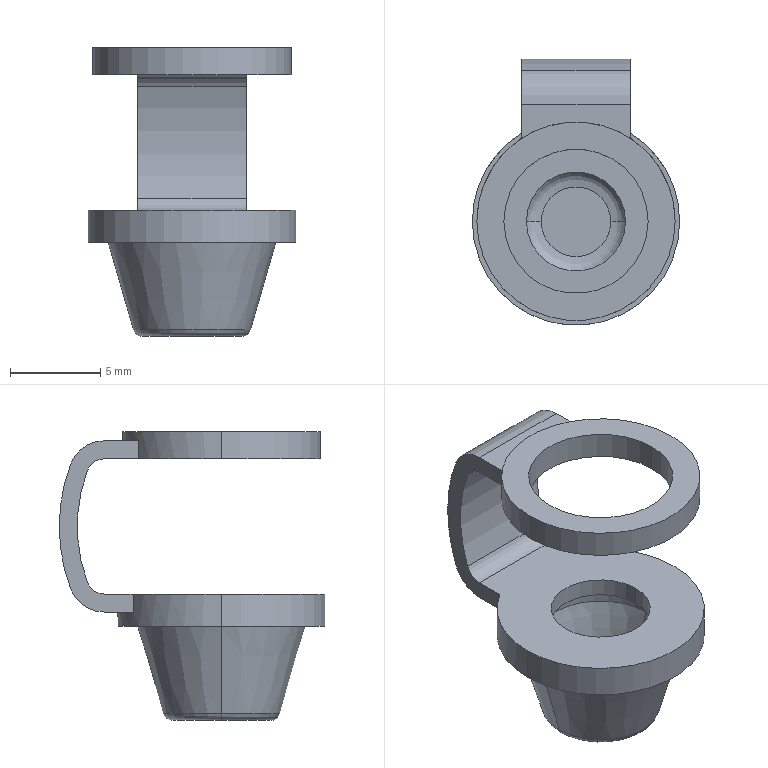Part | SolidWorks | features BaseBody 1 | 1 solid | 35 faces | box 11.5 x 14.75 x 16 mm | volume 426.893 mm3 | cylinder 16 | plane 11 | torus 4 | cone 4 | commonest cylinder face diameters 2 x2 4 x2 5.5 x2 7.1 x2 8 x2 11 x2
STEP:
#1=CARTESIAN_POINT('',(-5.5,0.,9.));
#2=VERTEX_POINT('',#1);
#3=CARTESIAN_POINT('',(-5.5,0.,7.5));
#4=VERTEX_POINT('',#3);
#5=CARTESIAN_POINT('',(-5.5,0.,2.274));
#6=DIRECTION('',(0.,0.,-1.));
#7=VECTOR('',#6,1000.);
#8=LINE('',#5,#7);
#9=EDGE_CURVE('',#2,#4,#8,.T.);
#10=ORIENTED_EDGE('',*,*,#9,.T.);
#11=CARTESIAN_POINT('',(5.5,0.,7.5));
#12=VERTEX_POINT('',#11);
#13=CARTESIAN_POINT('',(0.,0.,7.5));
#14=DIRECTION('',(0.,0.,1.));
#15=DIRECTION('',(1.,0.,0.));
#16=AXIS2_PLACEMENT_3D('',#13,#14,#15);
#17=CIRCLE('',#16,5.5);
#18=EDGE_CURVE('',#4,#12,#17,.T.);
#19=ORIENTED_EDGE('',*,*,#18,.T.);
#20=CARTESIAN_POINT('',(5.5,0.,9.));
#21=VERTEX_POINT('',#20);
#22=CARTESIAN_POINT('',(5.5,0.,2.274));
#23=DIRECTION('',(0.,0.,-1.));
#24=VECTOR('',#23,1000.);
#25=LINE('',#22,#24);
#26=EDGE_CURVE('',#21,#12,#25,.T.);
#27=ORIENTED_EDGE('',*,*,#26,.F.);
#28=CARTESIAN_POINT('',(0.,0.,9.));
#29=DIRECTION('',(0.,0.,1.));
#30=DIRECTION('',(1.,0.,0.));
#31=AXIS2_PLACEMENT_3D('',#28,#29,#30);
#32=CIRCLE('',#31,5.5);
#33=EDGE_CURVE('',#2,#21,#32,.T.);
#34=ORIENTED_EDGE('',*,*,#33,.F.);
#35=EDGE_LOOP('',(#10,#19,#27,#34));
#36=FACE_OUTER_BOUND('',#35,.T.);
#37=CARTESIAN_POINT('',(0.,0.,2.274));
#38=DIRECTION('',(0.,0.,-1.));
#39=DIRECTION('',(1.,0.,0.));
#40=AXIS2_PLACEMENT_3D('',#37,#38,#39);
#41=CYLINDRICAL_SURFACE('',#40,5.5);
#42=ADVANCED_FACE('',(#36),#41,.T.);
#43=CARTESIAN_POINT('',(4.,0.,9.));
#44=VERTEX_POINT('',#43);
#45=CARTESIAN_POINT('',(-4.,0.,9.));
#46=VERTEX_POINT('',#45);
#47=CARTESIAN_POINT('',(0.,0.,9.));
#48=DIRECTION('',(0.,0.,1.));
#49=DIRECTION('',(1.,0.,0.));
#50=AXIS2_PLACEMENT_3D('',#47,#48,#49);
#51=CIRCLE('',#50,4.);
#52=EDGE_CURVE('',#44,#46,#51,.T.);
#53=ORIENTED_EDGE('',*,*,#52,.F.);
#54=CARTESIAN_POINT('',(0.,0.,9.));
#55=DIRECTION('',(0.,0.,1.));
#56=DIRECTION('',(1.,0.,0.));
#57=AXIS2_PLACEMENT_3D('',#54,#55,#56);
#58=CIRCLE('',#57,4.);
#59=EDGE_CURVE('',#46,#44,#58,.T.);
#60=ORIENTED_EDGE('',*,*,#59,.F.);
#61=EDGE_LOOP('',(#53,#60));
#62=FACE_BOUND('',#61,.T.);
#63=CARTESIAN_POINT('',(0.,0.,9.));
#64=DIRECTION('',(0.,0.,1.));
#65=DIRECTION('',(1.,0.,0.));
#66=AXIS2_PLACEMENT_3D('',#63,#64,#65);
#67=CIRCLE('',#66,5.5);
#68=EDGE_CURVE('',#21,#2,#67,.T.);
#69=ORIENTED_EDGE('',*,*,#68,.T.);
#70=ORIENTED_EDGE('',*,*,#33,.T.);
#71=EDGE_LOOP('',(#69,#70));
#72=FACE_OUTER_BOUND('',#71,.T.);
#73=CARTESIAN_POINT('',(0.,5.5,9.));
#74=DIRECTION('',(0.,0.,-1.));
#75=DIRECTION('',(-1.,0.,0.));
#76=AXIS2_PLACEMENT_3D('',#73,#74,#75);
#77=PLANE('',#76);
#78=ADVANCED_FACE('',(#62,#72),#77,.F.);
#79=CARTESIAN_POINT('',(-4.,0.,7.5));
#80=VERTEX_POINT('',#79);
#81=CARTESIAN_POINT('',(-4.,0.,2.274));
#82=DIRECTION('',(0.,0.,-1.));
#83=VECTOR('',#82,1000.);
#84=LINE('',#81,#83);
#85=EDGE_CURVE('',#46,#80,#84,.T.);
#86=ORIENTED_EDGE('',*,*,#85,.T.);
#87=CARTESIAN_POINT('',(4.,0.,7.5));
#88=VERTEX_POINT('',#87);
#89=CARTESIAN_POINT('',(0.,0.,7.5));
#90=DIRECTION('',(0.,0.,1.));
#91=DIRECTION('',(1.,0.,0.));
#92=AXIS2_PLACEMENT_3D('',#89,#90,#91);
#93=CIRCLE('',#92,4.);
#94=EDGE_CURVE('',#88,#80,#93,.T.);
#95=ORIENTED_EDGE('',*,*,#94,.F.);
#96=CARTESIAN_POINT('',(4.,0.,2.274));
#97=DIRECTION('',(0.,0.,-1.));
#98=VECTOR('',#97,1000.);
#99=LINE('',#96,#98);
#100=EDGE_CURVE('',#44,#88,#99,.T.);
#101=ORIENTED_EDGE('',*,*,#100,.F.);
#102=ORIENTED_EDGE('',*,*,#52,.T.);
#103=EDGE_LOOP('',(#86,#95,#101,#102));
#104=FACE_OUTER_BOUND('',#103,.T.);
#105=CARTESIAN_POINT('',(0.,0.,2.274));
#106=DIRECTION('',(0.,0.,-1.));
#107=DIRECTION('',(1.,0.,0.));
#108=AXIS2_PLACEMENT_3D('',#105,#106,#107);
#109=CYLINDRICAL_SURFACE('',#108,4.);
#110=ADVANCED_FACE('',(#104),#109,.F.);
#111=CARTESIAN_POINT('',(-3.,6.5,0.));
#112=VERTEX_POINT('',#111);
#113=CARTESIAN_POINT('',(3.,6.5,0.));
#114=VERTEX_POINT('',#113);
#115=CARTESIAN_POINT('',(-3.,6.5,0.));
#116=DIRECTION('',(1.,0.,0.));
#117=VECTOR('',#116,1000.);
#118=LINE('',#115,#117);
#119=EDGE_CURVE('',#112,#114,#118,.T.);
#120=ORIENTED_EDGE('',*,*,#119,.T.);
#121=CARTESIAN_POINT('',(3.,7.436,0.648));
#122=VERTEX_POINT('',#121);
#123=CARTESIAN_POINT('',(3.,6.5,1.));
#124=DIRECTION('',(1.,0.,0.));
#125=DIRECTION('',(0.,0.,-1.));
#126=AXIS2_PLACEMENT_3D('',#123,#124,#125);
#127=CIRCLE('',#126,1.);
#128=EDGE_CURVE('',#114,#122,#127,.T.);
#129=ORIENTED_EDGE('',*,*,#128,.T.);
#130=CARTESIAN_POINT('',(-3.,7.436,0.648));
#131=VERTEX_POINT('',#130);
#132=CARTESIAN_POINT('',(-3.,7.436,0.648));
#133=DIRECTION('',(1.,0.,0.));
#134=VECTOR('',#133,1000.);
#135=LINE('',#132,#134);
#136=EDGE_CURVE('',#131,#122,#135,.T.);
#137=ORIENTED_EDGE('',*,*,#136,.F.);
#138=CARTESIAN_POINT('',(-3.,6.5,1.));
#139=DIRECTION('',(1.,0.,0.));
#140=DIRECTION('',(0.,0.,-1.));
#141=AXIS2_PLACEMENT_3D('',#138,#139,#140);
#142=CIRCLE('',#141,1.);
#143=EDGE_CURVE('',#112,#131,#142,.T.);
#144=ORIENTED_EDGE('',*,*,#143,.F.);
#145=EDGE_LOOP('',(#120,#129,#137,#144));
#146=FACE_OUTER_BOUND('',#145,.T.);
#147=CARTESIAN_POINT('',(0.,6.5,1.));
#148=DIRECTION('',(-1.,0.,0.));
#149=DIRECTION('',(0.,0.,-1.));
#150=AXIS2_PLACEMENT_3D('',#147,#148,#149);
#151=CYLINDRICAL_SURFACE('',#150,1.);
#152=ADVANCED_FACE('',(#146),#151,.F.);
#153=CARTESIAN_POINT('',(3.,6.5,-1.));
#154=VERTEX_POINT('',#153);
#155=CARTESIAN_POINT('',(-3.,6.5,-1.));
#156=VERTEX_POINT('',#155);
#157=CARTESIAN_POINT('',(-3.,6.5,-1.));
#158=DIRECTION('',(-1.,0.,0.));
#159=VECTOR('',#158,1000.);
#160=LINE('',#157,#159);
#161=EDGE_CURVE('',#154,#156,#160,.T.);
#162=ORIENTED_EDGE('',*,*,#161,.T.);
#163=CARTESIAN_POINT('',(-3.,8.372,0.296));
#164=VERTEX_POINT('',#163);
#165=CARTESIAN_POINT('',(-3.,6.5,1.));
#166=DIRECTION('',(1.,0.,0.));
#167=DIRECTION('',(0.,0.,-1.));
#168=AXIS2_PLACEMENT_3D('',#165,#166,#167);
#169=CIRCLE('',#168,2.);
#170=EDGE_CURVE('',#156,#164,#169,.T.);
#171=ORIENTED_EDGE('',*,*,#170,.T.);
#172=CARTESIAN_POINT('',(3.,8.372,0.296));
#173=VERTEX_POINT('',#172);
#174=CARTESIAN_POINT('',(-3.,8.372,0.296));
#175=DIRECTION('',(-1.,0.,0.));
#176=VECTOR('',#175,1000.);
#177=LINE('',#174,#176);
#178=EDGE_CURVE('',#173,#164,#177,.T.);
#179=ORIENTED_EDGE('',*,*,#178,.F.);
#180=CARTESIAN_POINT('',(3.,6.5,1.));
#181=DIRECTION('',(1.,0.,0.));
#182=DIRECTION('',(0.,0.,-1.));
#183=AXIS2_PLACEMENT_3D('',#180,#181,#182);
#184=CIRCLE('',#183,2.);
#185=EDGE_CURVE('',#154,#173,#184,.T.);
#186=ORIENTED_EDGE('',*,*,#185,.F.);
#187=EDGE_LOOP('',(#162,#171,#179,#186));
#188=FACE_OUTER_BOUND('',#187,.T.);
#189=CARTESIAN_POINT('',(0.,6.5,1.));
#190=DIRECTION('',(-1.,0.,0.));
#191=DIRECTION('',(0.,0.,-1.));
#192=AXIS2_PLACEMENT_3D('',#189,#190,#191);
#193=CYLINDRICAL_SURFACE('',#192,2.);
#194=ADVANCED_FACE('',(#188),#193,.T.);
#195=ORIENTED_EDGE('',*,*,#136,.T.);
#196=CARTESIAN_POINT('',(3.,7.436,6.852));
#197=VERTEX_POINT('',#196);
#198=CARTESIAN_POINT('',(3.,-0.8125,3.75));
#199=DIRECTION('',(1.,0.,0.));
#200=DIRECTION('',(0.,0.,-1.));
#201=AXIS2_PLACEMENT_3D('',#198,#199,#200);
#202=CIRCLE('',#201,8.812);
#203=EDGE_CURVE('',#122,#197,#202,.T.);
#204=ORIENTED_EDGE('',*,*,#203,.T.);
#205=CARTESIAN_POINT('',(-3.,7.436,6.852));
#206=VERTEX_POINT('',#205);
#207=CARTESIAN_POINT('',(-3.,7.436,6.852));
#208=DIRECTION('',(1.,0.,0.));
#209=VECTOR('',#208,1000.);
#210=LINE('',#207,#209);
#211=EDGE_CURVE('',#206,#197,#210,.T.);
#212=ORIENTED_EDGE('',*,*,#211,.F.);
#213=CARTESIAN_POINT('',(-3.,-0.8125,3.75));
#214=DIRECTION('',(1.,0.,0.));
#215=DIRECTION('',(0.,0.,-1.));
#216=AXIS2_PLACEMENT_3D('',#213,#214,#215);
#217=CIRCLE('',#216,8.812);
#218=EDGE_CURVE('',#131,#206,#217,.T.);
#219=ORIENTED_EDGE('',*,*,#218,.F.);
#220=EDGE_LOOP('',(#195,#204,#212,#219));
#221=FACE_OUTER_BOUND('',#220,.T.);
#222=CARTESIAN_POINT('',(0.,-0.8125,3.75));
#223=DIRECTION('',(-1.,0.,0.));
#224=DIRECTION('',(0.,0.,-1.));
#225=AXIS2_PLACEMENT_3D('',#222,#223,#224);
#226=CYLINDRICAL_SURFACE('',#225,8.812);
#227=ADVANCED_FACE('',(#221),#226,.F.);
#228=ORIENTED_EDGE('',*,*,#178,.T.);
#229=CARTESIAN_POINT('',(-3.,8.372,7.204));
#230=VERTEX_POINT('',#229);
#231=CARTESIAN_POINT('',(-3.,-0.8125,3.75));
#232=DIRECTION('',(1.,0.,0.));
#233=DIRECTION('',(0.,0.,-1.));
#234=AXIS2_PLACEMENT_3D('',#231,#232,#233);
#235=CIRCLE('',#234,9.812);
#236=EDGE_CURVE('',#164,#230,#235,.T.);
#237=ORIENTED_EDGE('',*,*,#236,.T.);
#238=CARTESIAN_POINT('',(3.,8.372,7.204));
#239=VERTEX_POINT('',#238);
#240=CARTESIAN_POINT('',(-3.,8.372,7.204));
#241=DIRECTION('',(-1.,0.,0.));
#242=VECTOR('',#241,1000.);
#243=LINE('',#240,#242);
#244=EDGE_CURVE('',#239,#230,#243,.T.);
#245=ORIENTED_EDGE('',*,*,#244,.F.);
#246=CARTESIAN_POINT('',(3.,-0.8125,3.75));
#247=DIRECTION('',(1.,0.,0.));
#248=DIRECTION('',(0.,0.,-1.));
#249=AXIS2_PLACEMENT_3D('',#246,#247,#248);
#250=CIRCLE('',#249,9.812);
#251=EDGE_CURVE('',#173,#239,#250,.T.);
#252=ORIENTED_EDGE('',*,*,#251,.F.);
#253=EDGE_LOOP('',(#228,#237,#245,#252));
#254=FACE_OUTER_BOUND('',#253,.T.);
#255=CARTESIAN_POINT('',(0.,-0.8125,3.75));
#256=DIRECTION('',(-1.,0.,0.));
#257=DIRECTION('',(0.,0.,-1.));
#258=AXIS2_PLACEMENT_3D('',#255,#256,#257);
#259=CYLINDRICAL_SURFACE('',#258,9.812);
#260=ADVANCED_FACE('',(#254),#259,.T.);
#261=ORIENTED_EDGE('',*,*,#211,.T.);
#262=CARTESIAN_POINT('',(3.,6.5,7.5));
#263=VERTEX_POINT('',#262);
#264=CARTESIAN_POINT('',(3.,6.5,6.5));
#265=DIRECTION('',(1.,0.,0.));
#266=DIRECTION('',(0.,0.,-1.));
#267=AXIS2_PLACEMENT_3D('',#264,#265,#266);
#268=CIRCLE('',#267,1.);
#269=EDGE_CURVE('',#197,#263,#268,.T.);
#270=ORIENTED_EDGE('',*,*,#269,.T.);
#271=CARTESIAN_POINT('',(-3.,6.5,7.5));
#272=VERTEX_POINT('',#271);
#273=CARTESIAN_POINT('',(-3.,6.5,7.5));
#274=DIRECTION('',(1.,0.,0.));
#275=VECTOR('',#274,1000.);
#276=LINE('',#273,#275);
#277=EDGE_CURVE('',#272,#263,#276,.T.);
#278=ORIENTED_EDGE('',*,*,#277,.F.);
#279=CARTESIAN_POINT('',(-3.,6.5,6.5));
#280=DIRECTION('',(1.,0.,0.));
#281=DIRECTION('',(0.,0.,-1.));
#282=AXIS2_PLACEMENT_3D('',#279,#280,#281);
#283=CIRCLE('',#282,1.);
#284=EDGE_CURVE('',#206,#272,#283,.T.);
#285=ORIENTED_EDGE('',*,*,#284,.F.);
#286=EDGE_LOOP('',(#261,#270,#278,#285));
#287=FACE_OUTER_BOUND('',#286,.T.);
#288=CARTESIAN_POINT('',(0.,6.5,6.5));
#289=DIRECTION('',(-1.,0.,0.));
#290=DIRECTION('',(0.,0.,-1.));
#291=AXIS2_PLACEMENT_3D('',#288,#289,#290);
#292=CYLINDRICAL_SURFACE('',#291,1.);
#293=ADVANCED_FACE('',(#287),#292,.F.);
#294=ORIENTED_EDGE('',*,*,#244,.T.);
#295=CARTESIAN_POINT('',(-3.,6.5,8.5));
#296=VERTEX_POINT('',#295);
#297=CARTESIAN_POINT('',(-3.,6.5,6.5));
#298=DIRECTION('',(1.,0.,0.));
#299=DIRECTION('',(0.,0.,-1.));
#300=AXIS2_PLACEMENT_3D('',#297,#298,#299);
#301=CIRCLE('',#300,2.);
#302=EDGE_CURVE('',#230,#296,#301,.T.);
#303=ORIENTED_EDGE('',*,*,#302,.T.);
#304=CARTESIAN_POINT('',(3.,6.5,8.5));
#305=VERTEX_POINT('',#304);
#306=CARTESIAN_POINT('',(-3.,6.5,8.5));
#307=DIRECTION('',(-1.,0.,0.));
#308=VECTOR('',#307,1000.);
#309=LINE('',#306,#308);
#310=EDGE_CURVE('',#305,#296,#309,.T.);
#311=ORIENTED_EDGE('',*,*,#310,.F.);
#312=CARTESIAN_POINT('',(3.,6.5,6.5));
#313=DIRECTION('',(1.,0.,0.));
#314=DIRECTION('',(0.,0.,-1.));
#315=AXIS2_PLACEMENT_3D('',#312,#313,#314);
#316=CIRCLE('',#315,2.);
#317=EDGE_CURVE('',#239,#305,#316,.T.);
#318=ORIENTED_EDGE('',*,*,#317,.F.);
#319=EDGE_LOOP('',(#294,#303,#311,#318));
#320=FACE_OUTER_BOUND('',#319,.T.);
#321=CARTESIAN_POINT('',(0.,6.5,6.5));
#322=DIRECTION('',(-1.,0.,0.));
#323=DIRECTION('',(0.,0.,-1.));
#324=AXIS2_PLACEMENT_3D('',#321,#322,#323);
#325=CYLINDRICAL_SURFACE('',#324,2.);
#326=ADVANCED_FACE('',(#320),#325,.T.);
#327=ORIENTED_EDGE('',*,*,#94,.T.);
#328=CARTESIAN_POINT('',(0.,0.,7.5));
#329=DIRECTION('',(0.,0.,1.));
#330=DIRECTION('',(1.,0.,0.));
#331=AXIS2_PLACEMENT_3D('',#328,#329,#330);
#332=CIRCLE('',#331,4.);
#333=EDGE_CURVE('',#80,#88,#332,.T.);
#334=ORIENTED_EDGE('',*,*,#333,.T.);
#335=EDGE_LOOP('',(#327,#334));
#336=FACE_BOUND('',#335,.T.);
#337=CARTESIAN_POINT('',(-3.,4.61,7.5));
#338=VERTEX_POINT('',#337);
#339=CARTESIAN_POINT('',(0.,0.,7.5));
#340=DIRECTION('',(0.,0.,1.));
#341=DIRECTION('',(1.,0.,0.));
#342=AXIS2_PLACEMENT_3D('',#339,#340,#341);
#343=CIRCLE('',#342,5.5);
#344=EDGE_CURVE('',#338,#4,#343,.T.);
#345=ORIENTED_EDGE('',*,*,#344,.F.);
#346=CARTESIAN_POINT('',(-3.,6.5,7.5));
#347=DIRECTION('',(0.,-1.,0.));
#348=VECTOR('',#347,1000.);
#349=LINE('',#346,#348);
#350=EDGE_CURVE('',#272,#338,#349,.T.);
#351=ORIENTED_EDGE('',*,*,#350,.F.);
#352=ORIENTED_EDGE('',*,*,#277,.T.);
#353=CARTESIAN_POINT('',(3.,4.61,7.5));
#354=VERTEX_POINT('',#353);
#355=CARTESIAN_POINT('',(3.,6.5,7.5));
#356=DIRECTION('',(0.,-1.,0.));
#357=VECTOR('',#356,1000.);
#358=LINE('',#355,#357);
#359=EDGE_CURVE('',#263,#354,#358,.T.);
#360=ORIENTED_EDGE('',*,*,#359,.T.);
#361=CARTESIAN_POINT('',(0.,0.,7.5));
#362=DIRECTION('',(0.,0.,1.));
#363=DIRECTION('',(1.,0.,0.));
#364=AXIS2_PLACEMENT_3D('',#361,#362,#363);
#365=CIRCLE('',#364,5.5);
#366=EDGE_CURVE('',#12,#354,#365,.T.);
#367=ORIENTED_EDGE('',*,*,#366,.F.);
#368=ORIENTED_EDGE('',*,*,#18,.F.);
#369=EDGE_LOOP('',(#345,#351,#352,#360,#367,#368));
#370=FACE_OUTER_BOUND('',#369,.T.);
#371=CARTESIAN_POINT('',(-3.,6.5,7.5));
#372=DIRECTION('',(0.,0.,1.));
#373=DIRECTION('',(1.,0.,0.));
#374=AXIS2_PLACEMENT_3D('',#371,#372,#373);
#375=PLANE('',#374);
#376=ADVANCED_FACE('',(#336,#370),#375,.F.);
#377=CARTESIAN_POINT('',(3.,4.905,-1.));
#378=VERTEX_POINT('',#377);
#379=CARTESIAN_POINT('',(-3.,4.905,-1.));
#380=VERTEX_POINT('',#379);
#381=CARTESIAN_POINT('',(0.,0.,-1.));
#382=DIRECTION('',(0.,0.,1.));
#383=DIRECTION('',(0.,-1.,0.));
#384=AXIS2_PLACEMENT_3D('',#381,#382,#383);
#385=CIRCLE('',#384,5.75);
#386=EDGE_CURVE('',#378,#380,#385,.T.);
#387=ORIENTED_EDGE('',*,*,#386,.T.);
#388=CARTESIAN_POINT('',(-3.,6.5,-1.));
#389=DIRECTION('',(0.,-1.,0.));
#390=VECTOR('',#389,1000.);
#391=LINE('',#388,#390);
#392=EDGE_CURVE('',#156,#380,#391,.T.);
#393=ORIENTED_EDGE('',*,*,#392,.F.);
#394=ORIENTED_EDGE('',*,*,#161,.F.);
#395=CARTESIAN_POINT('',(3.,6.5,-1.));
#396=DIRECTION('',(0.,-1.,0.));
#397=VECTOR('',#396,1000.);
#398=LINE('',#395,#397);
#399=EDGE_CURVE('',#154,#378,#398,.T.);
#400=ORIENTED_EDGE('',*,*,#399,.T.);
#401=EDGE_LOOP('',(#387,#393,#394,#400));
#402=FACE_OUTER_BOUND('',#401,.T.);
#403=CARTESIAN_POINT('',(-3.,6.5,-1.));
#404=DIRECTION('',(0.,0.,-1.));
#405=DIRECTION('',(-1.,0.,0.));
#406=AXIS2_PLACEMENT_3D('',#403,#404,#405);
#407=PLANE('',#406);
#408=ADVANCED_FACE('',(#402),#407,.T.);
#409=CARTESIAN_POINT('',(1.931,0.,-5.));
#410=VERTEX_POINT('',#409);
#411=CARTESIAN_POINT('',(-1.931,0.,-5.));
#412=VERTEX_POINT('',#411);
#413=CARTESIAN_POINT('',(0.,0.,-5.));
#414=DIRECTION('',(0.,0.,1.));
#415=DIRECTION('',(1.,0.,0.));
#416=AXIS2_PLACEMENT_3D('',#413,#414,#415);
#417=CIRCLE('',#416,1.931);
#418=EDGE_CURVE('',#410,#412,#417,.T.);
#419=ORIENTED_EDGE('',*,*,#418,.T.);
#420=CARTESIAN_POINT('',(0.,0.,-5.));
#421=DIRECTION('',(0.,0.,1.));
#422=DIRECTION('',(1.,0.,0.));
#423=AXIS2_PLACEMENT_3D('',#420,#421,#422);
#424=CIRCLE('',#423,1.931);
#425=EDGE_CURVE('',#412,#410,#424,.T.);
#426=ORIENTED_EDGE('',*,*,#425,.T.);
#427=EDGE_LOOP('',(#419,#426));
#428=FACE_OUTER_BOUND('',#427,.T.);
#429=CARTESIAN_POINT('',(0.,1.931,-5.));
#430=DIRECTION('',(0.,0.,-1.));
#431=DIRECTION('',(-1.,0.,0.));
#432=AXIS2_PLACEMENT_3D('',#429,#430,#431);
#433=PLANE('',#432);
#434=ADVANCED_FACE('',(#428),#433,.F.);
#435=CARTESIAN_POINT('',(-2.892,0.,-4.278));
#436=VERTEX_POINT('',#435);
#437=CARTESIAN_POINT('',(-1.931,0.,-4.));
#438=DIRECTION('',(0.,-1.,0.));
#439=DIRECTION('',(-1.,0.,0.));
#440=AXIS2_PLACEMENT_3D('',#437,#438,#439);
#441=CIRCLE('',#440,1.);
#442=EDGE_CURVE('',#436,#412,#441,.T.);
#443=ORIENTED_EDGE('',*,*,#442,.T.);
#444=ORIENTED_EDGE('',*,*,#418,.F.);
#445=CARTESIAN_POINT('',(2.892,0.,-4.278));
#446=VERTEX_POINT('',#445);
#447=CARTESIAN_POINT('',(1.931,0.,-4.));
#448=DIRECTION('',(0.,1.,0.));
#449=DIRECTION('',(1.,0.,0.));
#450=AXIS2_PLACEMENT_3D('',#447,#448,#449);
#451=CIRCLE('',#450,1.);
#452=EDGE_CURVE('',#446,#410,#451,.T.);
#453=ORIENTED_EDGE('',*,*,#452,.F.);
#454=CARTESIAN_POINT('',(0.,0.,-4.278));
#455=DIRECTION('',(0.,0.,1.));
#456=DIRECTION('',(1.,0.,0.));
#457=AXIS2_PLACEMENT_3D('',#454,#455,#456);
#458=CIRCLE('',#457,2.892);
#459=EDGE_CURVE('',#446,#436,#458,.T.);
#460=ORIENTED_EDGE('',*,*,#459,.T.);
#461=EDGE_LOOP('',(#443,#444,#453,#460));
#462=FACE_OUTER_BOUND('',#461,.T.);
#463=CARTESIAN_POINT('',(0.,0.,-4.));
#464=DIRECTION('',(0.,0.,-1.));
#465=DIRECTION('',(1.,0.,0.));
#466=AXIS2_PLACEMENT_3D('',#463,#464,#465);
#467=TOROIDAL_SURFACE('',#466,1.931,1.);
#468=ADVANCED_FACE('',(#462),#467,.F.);
#469=CARTESIAN_POINT('',(3.55,0.,-2.));
#470=VERTEX_POINT('',#469);
#471=CARTESIAN_POINT('',(2.892,0.,-4.278));
#472=DIRECTION('',(0.2777,0.,0.9607));
#473=VECTOR('',#472,1000.);
#474=LINE('',#471,#473);
#475=EDGE_CURVE('',#446,#470,#474,.T.);
#476=ORIENTED_EDGE('',*,*,#475,.T.);
#477=CARTESIAN_POINT('',(-3.55,0.,-2.));
#478=VERTEX_POINT('',#477);
#479=CARTESIAN_POINT('',(0.,0.,-2.));
#480=DIRECTION('',(0.,0.,1.));
#481=DIRECTION('',(1.,0.,0.));
#482=AXIS2_PLACEMENT_3D('',#479,#480,#481);
#483=CIRCLE('',#482,3.55);
#484=EDGE_CURVE('',#470,#478,#483,.T.);
#485=ORIENTED_EDGE('',*,*,#484,.T.);
#486=CARTESIAN_POINT('',(-2.892,0.,-4.278));
#487=DIRECTION('',(-0.2777,0.,0.9607));
#488=VECTOR('',#487,1000.);
#489=LINE('',#486,#488);
#490=EDGE_CURVE('',#436,#478,#489,.T.);
#491=ORIENTED_EDGE('',*,*,#490,.F.);
#492=ORIENTED_EDGE('',*,*,#459,.F.);
#493=EDGE_LOOP('',(#476,#485,#491,#492));
#494=FACE_OUTER_BOUND('',#493,.T.);
#495=CARTESIAN_POINT('',(0.,0.,-4.278));
#496=DIRECTION('',(0.,0.,1.));
#497=DIRECTION('',(-1.,0.,0.));
#498=AXIS2_PLACEMENT_3D('',#495,#496,#497);
#499=CONICAL_SURFACE('',#498,2.892,0.2814);
#500=ADVANCED_FACE('',(#494),#499,.F.);
#501=CARTESIAN_POINT('',(-3.55,0.,-1.));
#502=VERTEX_POINT('',#501);
#503=CARTESIAN_POINT('',(-3.55,0.,0.));
#504=DIRECTION('',(0.,0.,-1.));
#505=VECTOR('',#504,1000.);
#506=LINE('',#503,#505);
#507=EDGE_CURVE('',#502,#478,#506,.T.);
#508=ORIENTED_EDGE('',*,*,#507,.T.);
#509=ORIENTED_EDGE('',*,*,#484,.F.);
#510=CARTESIAN_POINT('',(3.55,0.,-1.));
#511=VERTEX_POINT('',#510);
#512=CARTESIAN_POINT('',(3.55,0.,0.));
#513=DIRECTION('',(0.,0.,-1.));
#514=VECTOR('',#513,1000.);
#515=LINE('',#512,#514);
#516=EDGE_CURVE('',#511,#470,#515,.T.);
#517=ORIENTED_EDGE('',*,*,#516,.F.);
#518=CARTESIAN_POINT('',(0.,0.,-1.));
#519=DIRECTION('',(0.,0.,1.));
#520=DIRECTION('',(1.,0.,0.));
#521=AXIS2_PLACEMENT_3D('',#518,#519,#520);
#522=CIRCLE('',#521,3.55);
#523=EDGE_CURVE('',#511,#502,#522,.T.);
#524=ORIENTED_EDGE('',*,*,#523,.T.);
#525=EDGE_LOOP('',(#508,#509,#517,#524));
#526=FACE_OUTER_BOUND('',#525,.T.);
#527=CARTESIAN_POINT('',(0.,0.,0.));
#528=DIRECTION('',(0.,0.,-1.));
#529=DIRECTION('',(1.,0.,0.));
#530=AXIS2_PLACEMENT_3D('',#527,#528,#529);
#531=CYLINDRICAL_SURFACE('',#530,3.55);
#532=ADVANCED_FACE('',(#526),#531,.F.);
#533=CARTESIAN_POINT('',(2.75,0.,-1.));
#534=VERTEX_POINT('',#533);
#535=CARTESIAN_POINT('',(-2.75,0.,-1.));
#536=VERTEX_POINT('',#535);
#537=CARTESIAN_POINT('',(0.,0.,-1.));
#538=DIRECTION('',(0.,0.,1.));
#539=DIRECTION('',(1.,0.,0.));
#540=AXIS2_PLACEMENT_3D('',#537,#538,#539);
#541=CIRCLE('',#540,2.75);
#542=EDGE_CURVE('',#534,#536,#541,.T.);
#543=ORIENTED_EDGE('',*,*,#542,.T.);
#544=CARTESIAN_POINT('',(0.,0.,-1.));
#545=DIRECTION('',(0.,0.,1.));
#546=DIRECTION('',(1.,0.,0.));
#547=AXIS2_PLACEMENT_3D('',#544,#545,#546);
#548=CIRCLE('',#547,2.75);
#549=EDGE_CURVE('',#536,#534,#548,.T.);
#550=ORIENTED_EDGE('',*,*,#549,.T.);
#551=EDGE_LOOP('',(#543,#550));
#552=FACE_BOUND('',#551,.T.);
#553=ORIENTED_EDGE('',*,*,#523,.F.);
#554=CARTESIAN_POINT('',(0.,0.,-1.));
#555=DIRECTION('',(0.,0.,1.));
#556=DIRECTION('',(1.,0.,0.));
#557=AXIS2_PLACEMENT_3D('',#554,#555,#556);
#558=CIRCLE('',#557,3.55);
#559=EDGE_CURVE('',#502,#511,#558,.T.);
#560=ORIENTED_EDGE('',*,*,#559,.F.);
#561=EDGE_LOOP('',(#553,#560));
#562=FACE_OUTER_BOUND('',#561,.T.);
#563=CARTESIAN_POINT('',(0.,2.75,-1.));
#564=DIRECTION('',(0.,0.,1.));
#565=DIRECTION('',(1.,0.,0.));
#566=AXIS2_PLACEMENT_3D('',#563,#564,#565);
#567=PLANE('',#566);
#568=ADVANCED_FACE('',(#552,#562),#567,.F.);
#569=CARTESIAN_POINT('',(-2.75,0.,0.));
#570=VERTEX_POINT('',#569);
#571=CARTESIAN_POINT('',(-2.75,0.,0.));
#572=DIRECTION('',(0.,0.,-1.));
#573=VECTOR('',#572,1000.);
#574=LINE('',#571,#573);
#575=EDGE_CURVE('',#570,#536,#574,.T.);
#576=ORIENTED_EDGE('',*,*,#575,.T.);
#577=ORIENTED_EDGE('',*,*,#542,.F.);
#578=CARTESIAN_POINT('',(2.75,0.,0.));
#579=VERTEX_POINT('',#578);
#580=CARTESIAN_POINT('',(2.75,0.,0.));
#581=DIRECTION('',(0.,0.,-1.));
#582=VECTOR('',#581,1000.);
#583=LINE('',#580,#582);
#584=EDGE_CURVE('',#579,#534,#583,.T.);
#585=ORIENTED_EDGE('',*,*,#584,.F.);
#586=CARTESIAN_POINT('',(0.,0.,0.));
#587=DIRECTION('',(0.,0.,1.));
#588=DIRECTION('',(1.,0.,0.));
#589=AXIS2_PLACEMENT_3D('',#586,#587,#588);
#590=CIRCLE('',#589,2.75);
#591=EDGE_CURVE('',#579,#570,#590,.T.);
#592=ORIENTED_EDGE('',*,*,#591,.T.);
#593=EDGE_LOOP('',(#576,#577,#585,#592));
#594=FACE_OUTER_BOUND('',#593,.T.);
#595=CARTESIAN_POINT('',(0.,0.,0.));
#596=DIRECTION('',(0.,0.,-1.));
#597=DIRECTION('',(1.,0.,0.));
#598=AXIS2_PLACEMENT_3D('',#595,#596,#597);
#599=CYLINDRICAL_SURFACE('',#598,2.75);
#600=ADVANCED_FACE('',(#594),#599,.F.);
#601=ORIENTED_EDGE('',*,*,#591,.F.);
#602=CARTESIAN_POINT('',(0.,0.,0.));
#603=DIRECTION('',(0.,0.,1.));
#604=DIRECTION('',(1.,0.,0.));
#605=AXIS2_PLACEMENT_3D('',#602,#603,#604);
#606=CIRCLE('',#605,2.75);
#607=EDGE_CURVE('',#570,#579,#606,.T.);
#608=ORIENTED_EDGE('',*,*,#607,.F.);
#609=EDGE_LOOP('',(#601,#608));
#610=FACE_BOUND('',#609,.T.);
#611=CARTESIAN_POINT('',(-3.,4.905,0.));
#612=VERTEX_POINT('',#611);
#613=CARTESIAN_POINT('',(-5.75,0.,0.));
#614=VERTEX_POINT('',#613);
#615=CARTESIAN_POINT('',(0.,0.,0.));
#616=DIRECTION('',(0.,0.,1.));
#617=DIRECTION('',(1.,0.,0.));
#618=AXIS2_PLACEMENT_3D('',#615,#616,#617);
#619=CIRCLE('',#618,5.75);
#620=EDGE_CURVE('',#612,#614,#619,.T.);
#621=ORIENTED_EDGE('',*,*,#620,.T.);
#622=CARTESIAN_POINT('',(5.75,0.,0.));
#623=VERTEX_POINT('',#622);
#624=CARTESIAN_POINT('',(0.,0.,0.));
#625=DIRECTION('',(0.,0.,1.));
#626=DIRECTION('',(1.,0.,0.));
#627=AXIS2_PLACEMENT_3D('',#624,#625,#626);
#628=CIRCLE('',#627,5.75);
#629=EDGE_CURVE('',#614,#623,#628,.T.);
#630=ORIENTED_EDGE('',*,*,#629,.T.);
#631=CARTESIAN_POINT('',(3.,4.905,0.));
#632=VERTEX_POINT('',#631);
#633=CARTESIAN_POINT('',(0.,0.,0.));
#634=DIRECTION('',(0.,0.,1.));
#635=DIRECTION('',(1.,0.,0.));
#636=AXIS2_PLACEMENT_3D('',#633,#634,#635);
#637=CIRCLE('',#636,5.75);
#638=EDGE_CURVE('',#623,#632,#637,.T.);
#639=ORIENTED_EDGE('',*,*,#638,.T.);
#640=CARTESIAN_POINT('',(3.,6.5,0.));
#641=DIRECTION('',(0.,-1.,0.));
#642=VECTOR('',#641,1000.);
#643=LINE('',#640,#642);
#644=EDGE_CURVE('',#114,#632,#643,.T.);
#645=ORIENTED_EDGE('',*,*,#644,.F.);
#646=ORIENTED_EDGE('',*,*,#119,.F.);
#647=CARTESIAN_POINT('',(-3.,6.5,0.));
#648=DIRECTION('',(0.,-1.,0.));
#649=VECTOR('',#648,1000.);
#650=LINE('',#647,#649);
#651=EDGE_CURVE('',#112,#612,#650,.T.);
#652=ORIENTED_EDGE('',*,*,#651,.T.);
#653=EDGE_LOOP('',(#621,#630,#639,#645,#646,#652));
#654=FACE_OUTER_BOUND('',#653,.T.);
#655=CARTESIAN_POINT('',(0.,2.75,0.));
#656=DIRECTION('',(0.,0.,-1.));
#657=DIRECTION('',(-1.,0.,0.));
#658=AXIS2_PLACEMENT_3D('',#655,#656,#657);
#659=PLANE('',#658);
#660=ADVANCED_FACE('',(#610,#654),#659,.F.);
#661=CARTESIAN_POINT('',(-5.75,0.,-1.8));
#662=VERTEX_POINT('',#661);
#663=CARTESIAN_POINT('',(-5.75,0.,0.));
#664=DIRECTION('',(0.,0.,-1.));
#665=VECTOR('',#664,1000.);
#666=LINE('',#663,#665);
#667=EDGE_CURVE('',#614,#662,#666,.T.);
#668=ORIENTED_EDGE('',*,*,#667,.T.);
#669=CARTESIAN_POINT('',(5.75,0.,-1.8));
#670=VERTEX_POINT('',#669);
#671=CARTESIAN_POINT('',(0.,0.,-1.8));
#672=DIRECTION('',(0.,0.,1.));
#673=DIRECTION('',(1.,0.,0.));
#674=AXIS2_PLACEMENT_3D('',#671,#672,#673);
#675=CIRCLE('',#674,5.75);
#676=EDGE_CURVE('',#662,#670,#675,.T.);
#677=ORIENTED_EDGE('',*,*,#676,.T.);
#678=CARTESIAN_POINT('',(5.75,0.,0.));
#679=DIRECTION('',(0.,0.,-1.));
#680=VECTOR('',#679,1000.);
#681=LINE('',#678,#680);
#682=EDGE_CURVE('',#623,#670,#681,.T.);
#683=ORIENTED_EDGE('',*,*,#682,.F.);
#684=ORIENTED_EDGE('',*,*,#629,.F.);
#685=EDGE_LOOP('',(#668,#677,#683,#684));
#686=FACE_OUTER_BOUND('',#685,.T.);
#687=CARTESIAN_POINT('',(0.,0.,0.));
#688=DIRECTION('',(0.,0.,-1.));
#689=DIRECTION('',(1.,0.,0.));
#690=AXIS2_PLACEMENT_3D('',#687,#688,#689);
#691=CYLINDRICAL_SURFACE('',#690,5.75);
#692=ADVANCED_FACE('',(#686),#691,.T.);
#693=CARTESIAN_POINT('',(-4.649,0.,-1.8));
#694=VERTEX_POINT('',#693);
#695=CARTESIAN_POINT('',(4.649,0.,-1.8));
#696=VERTEX_POINT('',#695);
#697=CARTESIAN_POINT('',(0.,0.,-1.8));
#698=DIRECTION('',(0.,0.,1.));
#699=DIRECTION('',(1.,0.,0.));
#700=AXIS2_PLACEMENT_3D('',#697,#698,#699);
#701=CIRCLE('',#700,4.649);
#702=EDGE_CURVE('',#694,#696,#701,.T.);
#703=ORIENTED_EDGE('',*,*,#702,.T.);
#704=CARTESIAN_POINT('',(0.,0.,-1.8));
#705=DIRECTION('',(0.,0.,1.));
#706=DIRECTION('',(1.,0.,0.));
#707=AXIS2_PLACEMENT_3D('',#704,#705,#706);
#708=CIRCLE('',#707,4.649);
#709=EDGE_CURVE('',#696,#694,#708,.T.);
#710=ORIENTED_EDGE('',*,*,#709,.T.);
#711=EDGE_LOOP('',(#703,#710));
#712=FACE_BOUND('',#711,.T.);
#713=CARTESIAN_POINT('',(0.,0.,-1.8));
#714=DIRECTION('',(0.,0.,1.));
#715=DIRECTION('',(1.,0.,0.));
#716=AXIS2_PLACEMENT_3D('',#713,#714,#715);
#717=CIRCLE('',#716,5.75);
#718=EDGE_CURVE('',#670,#662,#717,.T.);
#719=ORIENTED_EDGE('',*,*,#718,.F.);
#720=ORIENTED_EDGE('',*,*,#676,.F.);
#721=EDGE_LOOP('',(#719,#720));
#722=FACE_OUTER_BOUND('',#721,.T.);
#723=CARTESIAN_POINT('',(0.,5.75,-1.8));
#724=DIRECTION('',(0.,0.,1.));
#725=DIRECTION('',(1.,0.,0.));
#726=AXIS2_PLACEMENT_3D('',#723,#724,#725);
#727=PLANE('',#726);
#728=ADVANCED_FACE('',(#712,#722),#727,.F.);
#729=CARTESIAN_POINT('',(3.25,0.,-6.639));
#730=VERTEX_POINT('',#729);
#731=CARTESIAN_POINT('',(4.649,0.,-1.8));
#732=DIRECTION('',(0.2777,0.,0.9607));
#733=VECTOR('',#732,1000.);
#734=LINE('',#731,#733);
#735=EDGE_CURVE('',#730,#696,#734,.T.);
#736=ORIENTED_EDGE('',*,*,#735,.T.);
#737=ORIENTED_EDGE('',*,*,#702,.F.);
#738=CARTESIAN_POINT('',(-3.25,0.,-6.639));
#739=VERTEX_POINT('',#738);
#740=CARTESIAN_POINT('',(-4.649,0.,-1.8));
#741=DIRECTION('',(-0.2777,0.,0.9607));
#742=VECTOR('',#741,1000.);
#743=LINE('',#740,#742);
#744=EDGE_CURVE('',#739,#694,#743,.T.);
#745=ORIENTED_EDGE('',*,*,#744,.F.);
#746=CARTESIAN_POINT('',(0.,0.,-6.639));
#747=DIRECTION('',(0.,0.,1.));
#748=DIRECTION('',(1.,0.,0.));
#749=AXIS2_PLACEMENT_3D('',#746,#747,#748);
#750=CIRCLE('',#749,3.25);
#751=EDGE_CURVE('',#739,#730,#750,.T.);
#752=ORIENTED_EDGE('',*,*,#751,.T.);
#753=EDGE_LOOP('',(#736,#737,#745,#752));
#754=FACE_OUTER_BOUND('',#753,.T.);
#755=CARTESIAN_POINT('',(0.,0.,-1.8));
#756=DIRECTION('',(0.,0.,1.));
#757=DIRECTION('',(-1.,0.,0.));
#758=AXIS2_PLACEMENT_3D('',#755,#756,#757);
#759=CONICAL_SURFACE('',#758,4.649,0.2814);
#760=ADVANCED_FACE('',(#754),#759,.T.);
#761=CARTESIAN_POINT('',(-2.77,0.,-7.));
#762=VERTEX_POINT('',#761);
#763=CARTESIAN_POINT('',(-2.77,0.,-6.5));
#764=DIRECTION('',(0.,-1.,0.));
#765=DIRECTION('',(-1.,0.,0.));
#766=AXIS2_PLACEMENT_3D('',#763,#764,#765);
#767=CIRCLE('',#766,0.5);
#768=EDGE_CURVE('',#739,#762,#767,.T.);
#769=ORIENTED_EDGE('',*,*,#768,.T.);
#770=CARTESIAN_POINT('',(2.77,0.,-7.));
#771=VERTEX_POINT('',#770);
#772=CARTESIAN_POINT('',(0.,0.,-7.));
#773=DIRECTION('',(0.,0.,1.));
#774=DIRECTION('',(1.,0.,0.));
#775=AXIS2_PLACEMENT_3D('',#772,#773,#774);
#776=CIRCLE('',#775,2.77);
#777=EDGE_CURVE('',#762,#771,#776,.T.);
#778=ORIENTED_EDGE('',*,*,#777,.T.);
#779=CARTESIAN_POINT('',(2.77,0.,-6.5));
#780=DIRECTION('',(0.,1.,0.));
#781=DIRECTION('',(1.,0.,0.));
#782=AXIS2_PLACEMENT_3D('',#779,#780,#781);
#783=CIRCLE('',#782,0.5);
#784=EDGE_CURVE('',#730,#771,#783,.T.);
#785=ORIENTED_EDGE('',*,*,#784,.F.);
#786=ORIENTED_EDGE('',*,*,#751,.F.);
#787=EDGE_LOOP('',(#769,#778,#785,#786));
#788=FACE_OUTER_BOUND('',#787,.T.);
#789=CARTESIAN_POINT('',(0.,0.,-6.5));
#790=DIRECTION('',(0.,0.,-1.));
#791=DIRECTION('',(1.,0.,0.));
#792=AXIS2_PLACEMENT_3D('',#789,#790,#791);
#793=TOROIDAL_SURFACE('',#792,2.77,0.5);
#794=ADVANCED_FACE('',(#788),#793,.T.);
#795=CARTESIAN_POINT('',(0.,0.,-7.));
#796=DIRECTION('',(0.,0.,1.));
#797=DIRECTION('',(1.,0.,0.));
#798=AXIS2_PLACEMENT_3D('',#795,#796,#797);
#799=CIRCLE('',#798,2.77);
#800=EDGE_CURVE('',#771,#762,#799,.T.);
#801=ORIENTED_EDGE('',*,*,#800,.F.);
#802=ORIENTED_EDGE('',*,*,#777,.F.);
#803=EDGE_LOOP('',(#801,#802));
#804=FACE_OUTER_BOUND('',#803,.T.);
#805=CARTESIAN_POINT('',(0.,2.77,-7.));
#806=DIRECTION('',(0.,0.,1.));
#807=DIRECTION('',(1.,0.,0.));
#808=AXIS2_PLACEMENT_3D('',#805,#806,#807);
#809=PLANE('',#808);
#810=ADVANCED_FACE('',(#804),#809,.F.);
#811=CARTESIAN_POINT('',(-3.,4.61,8.5));
#812=VERTEX_POINT('',#811);
#813=CARTESIAN_POINT('',(3.,4.61,8.5));
#814=VERTEX_POINT('',#813);
#815=CARTESIAN_POINT('',(0.,0.,8.5));
#816=DIRECTION('',(0.,0.,-1.));
#817=DIRECTION('',(1.,0.,0.));
#818=AXIS2_PLACEMENT_3D('',#815,#816,#817);
#819=CIRCLE('',#818,5.5);
#820=EDGE_CURVE('',#812,#814,#819,.T.);
#821=ORIENTED_EDGE('',*,*,#820,.T.);
#822=CARTESIAN_POINT('',(3.,6.5,8.5));
#823=DIRECTION('',(0.,-1.,0.));
#824=VECTOR('',#823,1000.);
#825=LINE('',#822,#824);
#826=EDGE_CURVE('',#305,#814,#825,.T.);
#827=ORIENTED_EDGE('',*,*,#826,.F.);
#828=ORIENTED_EDGE('',*,*,#310,.T.);
#829=CARTESIAN_POINT('',(-3.,6.5,8.5));
#830=DIRECTION('',(0.,-1.,0.));
#831=VECTOR('',#830,1000.);
#832=LINE('',#829,#831);
#833=EDGE_CURVE('',#296,#812,#832,.T.);
#834=ORIENTED_EDGE('',*,*,#833,.T.);
#835=EDGE_LOOP('',(#821,#827,#828,#834));
#836=FACE_OUTER_BOUND('',#835,.T.);
#837=CARTESIAN_POINT('',(-3.,6.5,8.5));
#838=DIRECTION('',(0.,0.,-1.));
#839=DIRECTION('',(-1.,0.,0.));
#840=AXIS2_PLACEMENT_3D('',#837,#838,#839);
#841=PLANE('',#840);
#842=ADVANCED_FACE('',(#836),#841,.F.);
#843=ORIENTED_EDGE('',*,*,#359,.F.);
#844=ORIENTED_EDGE('',*,*,#269,.F.);
#845=ORIENTED_EDGE('',*,*,#203,.F.);
#846=ORIENTED_EDGE('',*,*,#128,.F.);
#847=ORIENTED_EDGE('',*,*,#644,.T.);
#848=CARTESIAN_POINT('',(3.,4.905,0.));
#849=DIRECTION('',(0.,0.,-1.));
#850=VECTOR('',#849,1000.);
#851=LINE('',#848,#850);
#852=EDGE_CURVE('',#632,#378,#851,.T.);
#853=ORIENTED_EDGE('',*,*,#852,.T.);
#854=ORIENTED_EDGE('',*,*,#399,.F.);
#855=ORIENTED_EDGE('',*,*,#185,.T.);
#856=ORIENTED_EDGE('',*,*,#251,.T.);
#857=ORIENTED_EDGE('',*,*,#317,.T.);
#858=ORIENTED_EDGE('',*,*,#826,.T.);
#859=CARTESIAN_POINT('',(3.,4.61,2.274));
#860=DIRECTION('',(0.,0.,1.));
#861=VECTOR('',#860,1000.);
#862=LINE('',#859,#861);
#863=EDGE_CURVE('',#354,#814,#862,.T.);
#864=ORIENTED_EDGE('',*,*,#863,.F.);
#865=EDGE_LOOP('',(#843,#844,#845,#846,#847,#853,#854,#855,#856,#857,#858,#864));
#866=FACE_OUTER_BOUND('',#865,.T.);
#867=CARTESIAN_POINT('',(3.,6.5,-1.));
#868=DIRECTION('',(1.,0.,0.));
#869=DIRECTION('',(0.,0.,-1.));
#870=AXIS2_PLACEMENT_3D('',#867,#868,#869);
#871=PLANE('',#870);
#872=ADVANCED_FACE('',(#866),#871,.T.);
#873=ORIENTED_EDGE('',*,*,#833,.F.);
#874=ORIENTED_EDGE('',*,*,#302,.F.);
#875=ORIENTED_EDGE('',*,*,#236,.F.);
#876=ORIENTED_EDGE('',*,*,#170,.F.);
#877=ORIENTED_EDGE('',*,*,#392,.T.);
#878=CARTESIAN_POINT('',(-3.,4.905,0.));
#879=DIRECTION('',(0.,0.,1.));
#880=VECTOR('',#879,1000.);
#881=LINE('',#878,#880);
#882=EDGE_CURVE('',#380,#612,#881,.T.);
#883=ORIENTED_EDGE('',*,*,#882,.T.);
#884=ORIENTED_EDGE('',*,*,#651,.F.);
#885=ORIENTED_EDGE('',*,*,#143,.T.);
#886=ORIENTED_EDGE('',*,*,#218,.T.);
#887=ORIENTED_EDGE('',*,*,#284,.T.);
#888=ORIENTED_EDGE('',*,*,#350,.T.);
#889=CARTESIAN_POINT('',(-3.,4.61,2.274));
#890=DIRECTION('',(0.,0.,-1.));
#891=VECTOR('',#890,1000.);
#892=LINE('',#889,#891);
#893=EDGE_CURVE('',#812,#338,#892,.T.);
#894=ORIENTED_EDGE('',*,*,#893,.F.);
#895=EDGE_LOOP('',(#873,#874,#875,#876,#877,#883,#884,#885,#886,#887,#888,#894));
#896=FACE_OUTER_BOUND('',#895,.T.);
#897=CARTESIAN_POINT('',(-3.,6.5,-1.));
#898=DIRECTION('',(-1.,0.,0.));
#899=DIRECTION('',(0.,1.,0.));
#900=AXIS2_PLACEMENT_3D('',#897,#898,#899);
#901=PLANE('',#900);
#902=ADVANCED_FACE('',(#896),#901,.T.);
#903=CARTESIAN_POINT('',(0.,0.,-6.639));
#904=DIRECTION('',(0.,0.,1.));
#905=DIRECTION('',(1.,0.,0.));
#906=AXIS2_PLACEMENT_3D('',#903,#904,#905);
#907=CIRCLE('',#906,3.25);
#908=EDGE_CURVE('',#730,#739,#907,.T.);
#909=ORIENTED_EDGE('',*,*,#908,.F.);
#910=ORIENTED_EDGE('',*,*,#784,.T.);
#911=ORIENTED_EDGE('',*,*,#800,.T.);
#912=ORIENTED_EDGE('',*,*,#768,.F.);
#913=EDGE_LOOP('',(#909,#910,#911,#912));
#914=FACE_OUTER_BOUND('',#913,.T.);
#915=CARTESIAN_POINT('',(0.,0.,-6.5));
#916=DIRECTION('',(0.,0.,-1.));
#917=DIRECTION('',(1.,0.,0.));
#918=AXIS2_PLACEMENT_3D('',#915,#916,#917);
#919=TOROIDAL_SURFACE('',#918,2.77,0.5);
#920=ADVANCED_FACE('',(#914),#919,.T.);
#921=ORIENTED_EDGE('',*,*,#908,.T.);
#922=ORIENTED_EDGE('',*,*,#744,.T.);
#923=ORIENTED_EDGE('',*,*,#709,.F.);
#924=ORIENTED_EDGE('',*,*,#735,.F.);
#925=EDGE_LOOP('',(#921,#922,#923,#924));
#926=FACE_OUTER_BOUND('',#925,.T.);
#927=CARTESIAN_POINT('',(0.,0.,-1.8));
#928=DIRECTION('',(0.,0.,1.));
#929=DIRECTION('',(-1.,0.,0.));
#930=AXIS2_PLACEMENT_3D('',#927,#928,#929);
#931=CONICAL_SURFACE('',#930,4.649,0.2814);
#932=ADVANCED_FACE('',(#926),#931,.T.);
#933=ORIENTED_EDGE('',*,*,#620,.F.);
#934=ORIENTED_EDGE('',*,*,#882,.F.);
#935=ORIENTED_EDGE('',*,*,#386,.F.);
#936=ORIENTED_EDGE('',*,*,#852,.F.);
#937=ORIENTED_EDGE('',*,*,#638,.F.);
#938=ORIENTED_EDGE('',*,*,#682,.T.);
#939=ORIENTED_EDGE('',*,*,#718,.T.);
#940=ORIENTED_EDGE('',*,*,#667,.F.);
#941=EDGE_LOOP('',(#933,#934,#935,#936,#937,#938,#939,#940));
#942=FACE_OUTER_BOUND('',#941,.T.);
#943=CARTESIAN_POINT('',(0.,0.,0.));
#944=DIRECTION('',(0.,0.,-1.));
#945=DIRECTION('',(1.,0.,0.));
#946=AXIS2_PLACEMENT_3D('',#943,#944,#945);
#947=CYLINDRICAL_SURFACE('',#946,5.75);
#948=ADVANCED_FACE('',(#942),#947,.T.);
#949=ORIENTED_EDGE('',*,*,#607,.T.);
#950=ORIENTED_EDGE('',*,*,#584,.T.);
#951=ORIENTED_EDGE('',*,*,#549,.F.);
#952=ORIENTED_EDGE('',*,*,#575,.F.);
#953=EDGE_LOOP('',(#949,#950,#951,#952));
#954=FACE_OUTER_BOUND('',#953,.T.);
#955=CARTESIAN_POINT('',(0.,0.,0.));
#956=DIRECTION('',(0.,0.,-1.));
#957=DIRECTION('',(1.,0.,0.));
#958=AXIS2_PLACEMENT_3D('',#955,#956,#957);
#959=CYLINDRICAL_SURFACE('',#958,2.75);
#960=ADVANCED_FACE('',(#954),#959,.F.);
#961=ORIENTED_EDGE('',*,*,#559,.T.);
#962=ORIENTED_EDGE('',*,*,#516,.T.);
#963=CARTESIAN_POINT('',(0.,0.,-2.));
#964=DIRECTION('',(0.,0.,1.));
#965=DIRECTION('',(1.,0.,0.));
#966=AXIS2_PLACEMENT_3D('',#963,#964,#965);
#967=CIRCLE('',#966,3.55);
#968=EDGE_CURVE('',#478,#470,#967,.T.);
#969=ORIENTED_EDGE('',*,*,#968,.F.);
#970=ORIENTED_EDGE('',*,*,#507,.F.);
#971=EDGE_LOOP('',(#961,#962,#969,#970));
#972=FACE_OUTER_BOUND('',#971,.T.);
#973=CARTESIAN_POINT('',(0.,0.,0.));
#974=DIRECTION('',(0.,0.,-1.));
#975=DIRECTION('',(1.,0.,0.));
#976=AXIS2_PLACEMENT_3D('',#973,#974,#975);
#977=CYLINDRICAL_SURFACE('',#976,3.55);
#978=ADVANCED_FACE('',(#972),#977,.F.);
#979=CARTESIAN_POINT('',(0.,0.,-4.278));
#980=DIRECTION('',(0.,0.,1.));
#981=DIRECTION('',(1.,0.,0.));
#982=AXIS2_PLACEMENT_3D('',#979,#980,#981);
#983=CIRCLE('',#982,2.892);
#984=EDGE_CURVE('',#436,#446,#983,.T.);
#985=ORIENTED_EDGE('',*,*,#984,.F.);
#986=ORIENTED_EDGE('',*,*,#490,.T.);
#987=ORIENTED_EDGE('',*,*,#968,.T.);
#988=ORIENTED_EDGE('',*,*,#475,.F.);
#989=EDGE_LOOP('',(#985,#986,#987,#988));
#990=FACE_OUTER_BOUND('',#989,.T.);
#991=CARTESIAN_POINT('',(0.,0.,-4.278));
#992=DIRECTION('',(0.,0.,1.));
#993=DIRECTION('',(-1.,0.,0.));
#994=AXIS2_PLACEMENT_3D('',#991,#992,#993);
#995=CONICAL_SURFACE('',#994,2.892,0.2814);
#996=ADVANCED_FACE('',(#990),#995,.F.);
#997=ORIENTED_EDGE('',*,*,#984,.T.);
#998=ORIENTED_EDGE('',*,*,#452,.T.);
#999=ORIENTED_EDGE('',*,*,#425,.F.);
#1000=ORIENTED_EDGE('',*,*,#442,.F.);
#1001=EDGE_LOOP('',(#997,#998,#999,#1000));
#1002=FACE_OUTER_BOUND('',#1001,.T.);
#1003=CARTESIAN_POINT('',(0.,0.,-4.));
#1004=DIRECTION('',(0.,0.,-1.));
#1005=DIRECTION('',(1.,0.,0.));
#1006=AXIS2_PLACEMENT_3D('',#1003,#1004,#1005);
#1007=TOROIDAL_SURFACE('',#1006,1.931,1.);
#1008=ADVANCED_FACE('',(#1002),#1007,.F.);
#1009=ORIENTED_EDGE('',*,*,#59,.T.);
#1010=ORIENTED_EDGE('',*,*,#100,.T.);
#1011=ORIENTED_EDGE('',*,*,#333,.F.);
#1012=ORIENTED_EDGE('',*,*,#85,.F.);
#1013=EDGE_LOOP('',(#1009,#1010,#1011,#1012));
#1014=FACE_OUTER_BOUND('',#1013,.T.);
#1015=CARTESIAN_POINT('',(0.,0.,2.274));
#1016=DIRECTION('',(0.,0.,-1.));
#1017=DIRECTION('',(1.,0.,0.));
#1018=AXIS2_PLACEMENT_3D('',#1015,#1016,#1017);
#1019=CYLINDRICAL_SURFACE('',#1018,4.);
#1020=ADVANCED_FACE('',(#1014),#1019,.F.);
#1021=ORIENTED_EDGE('',*,*,#68,.F.);
#1022=ORIENTED_EDGE('',*,*,#26,.T.);
#1023=ORIENTED_EDGE('',*,*,#366,.T.);
#1024=ORIENTED_EDGE('',*,*,#863,.T.);
#1025=ORIENTED_EDGE('',*,*,#820,.F.);
#1026=ORIENTED_EDGE('',*,*,#893,.T.);
#1027=ORIENTED_EDGE('',*,*,#344,.T.);
#1028=ORIENTED_EDGE('',*,*,#9,.F.);
#1029=EDGE_LOOP('',(#1021,#1022,#1023,#1024,#1025,#1026,#1027,#1028));
#1030=FACE_OUTER_BOUND('',#1029,.T.);
#1031=CARTESIAN_POINT('',(0.,0.,2.274));
#1032=DIRECTION('',(0.,0.,-1.));
#1033=DIRECTION('',(1.,0.,0.));
#1034=AXIS2_PLACEMENT_3D('',#1031,#1032,#1033);
#1035=CYLINDRICAL_SURFACE('',#1034,5.5);
#1036=ADVANCED_FACE('',(#1030),#1035,.T.);
#1037=CLOSED_SHELL('',(#42,#78,#110,#152,#194,#227,#260,#293,#326,#376,#408,#434,#468,#500,#532,#568,#600,#660,#692,#728,#760,#794,#810,#842,#872,#902,#920,#932,#948,#960,#978,#996,#1008,#1020,#1036));
#1038=MANIFOLD_SOLID_BREP('',#1037);
#1039=CARTESIAN_POINT('',(0.,0.,0.));
#1040=DIRECTION('',(0.,0.,1.));
#1041=DIRECTION('',(1.,0.,0.));
#1042=AXIS2_PLACEMENT_3D('',#1039,#1040,#1041);
#1043=(LENGTH_UNIT()NAMED_UNIT(*)SI_UNIT(.MILLI.,.METRE.));
#1044=UNCERTAINTY_MEASURE_WITH_UNIT(LENGTH_MEASURE(0.00001),#1043,'','');
#1045=(NAMED_UNIT(*)PLANE_ANGLE_UNIT()SI_UNIT($,.RADIAN.));
#1046=(NAMED_UNIT(*)SI_UNIT($,.STERADIAN.)SOLID_ANGLE_UNIT());
#1047=(GEOMETRIC_REPRESENTATION_CONTEXT(3)GLOBAL_UNCERTAINTY_ASSIGNED_CONTEXT((#1044))GLOBAL_UNIT_ASSIGNED_CONTEXT((#1043,#1045,#1046))REPRESENTATION_CONTEXT('',''));
#1048=ADVANCED_BREP_SHAPE_REPRESENTATION('',(#1038,#1042),#1047);